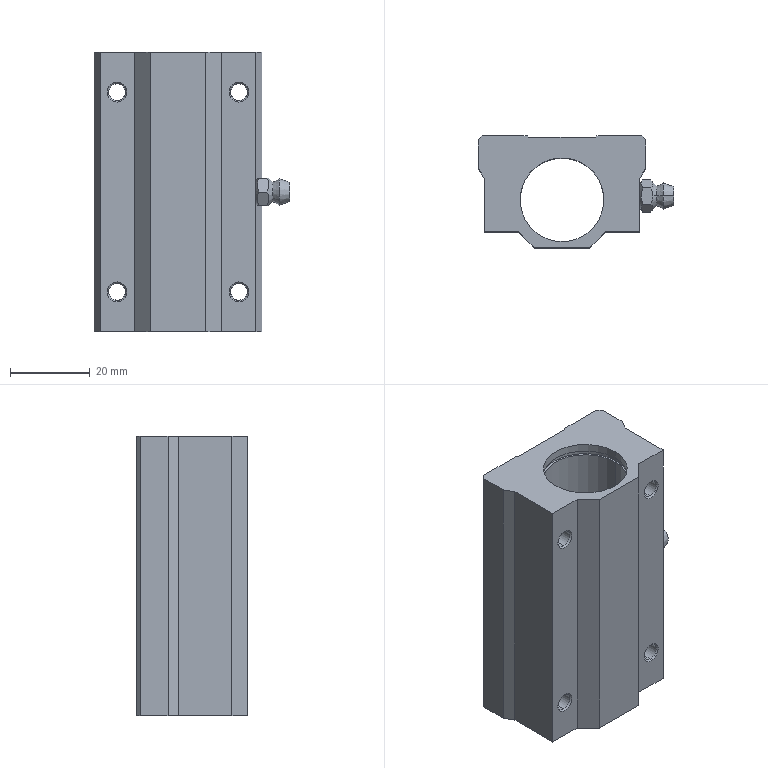Part | STEP file | LHBBW12body_Default | 1 solid | 85 faces | box 49 x 28 x 70 mm | volume 46534 mm3 | plane 35 | cylinder 26 | cone 24 | commonest cylinder face diameters 4.134 x8 4.3 x8 21 x6 22 x4